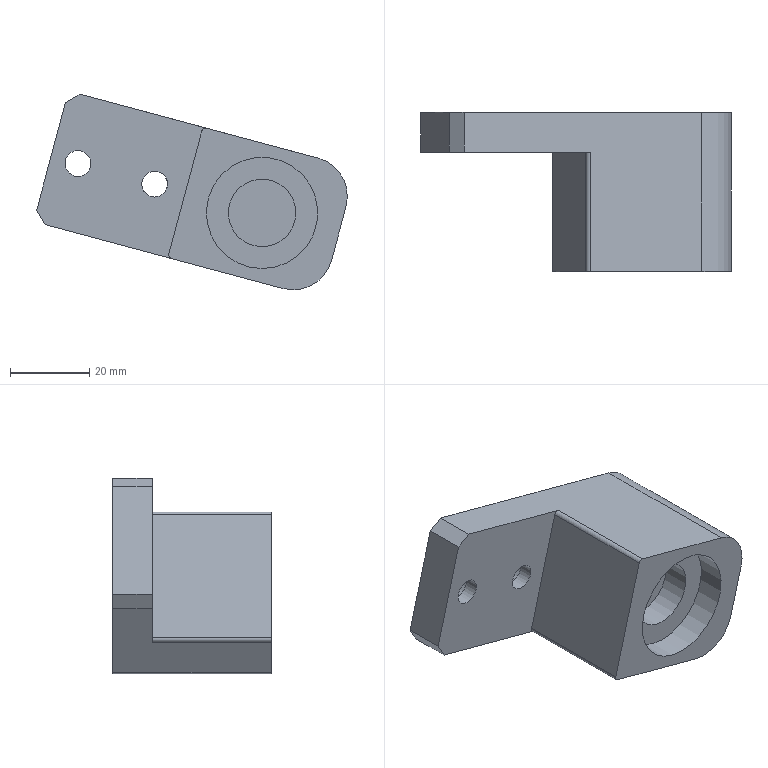CAM job | NX | 3+2 milling, drilling | part box 78.22 x 40 x 49.229 mm | stock box 86.333 x 45 x 54.513 mm
Tools:
number,name,description,diameter,corner_radius,flute_length,length,flutes
6,D6,平底铣刀-粗,6.0,0.0,25.0,75.0,2
9,D10,平底铣刀-粗,10.0,0.0,35.0,75.0,2
7,D6-J,平底铣刀-精,6.0,0.0,25.0,75.0,2
10,D10-J,平底铣刀-精,10.0,0.0,35.0,75.0,2
1,D80R0.8飞刀,圆鼻刀-粗,80.0,0.8,50.0,75.0,2
1,D80R0.8飞刀-J,圆鼻刀-精,80.0,0.8,50.0,75.0,2
2,D6倒角刀,倒角刀,6.0,0.0,3.0,25.0,2
17,ZT6.5,钻头,6.5,0.0,35.0,50.0,2
Operations:
program,operation,operation_type,tool,method,geometry_group,spindle_rpm,surface_speed,feed_per_tooth,feed_cut,feed_plunge,cut_length_mm,path_length_mm,cut_time_min,machine_time_min
B,底壁铣飞面一刀开粗_COPY,VolumeBased25DMillingOperation,D80R0.8飞刀,分层开粗-切深K-步距G,W-B,2800.0,703.696,0.5357,3000.0,100.0,1649.091,3281.618,0.5497,0.7129
B,底壁铣飞面一刀精光_COPY,VolumeBased25DMillingOperation,D80R0.8飞刀-J,侧刃精光-切深K-步距G,W-B,4000.0,1005.28,0.125,1000.0,100.0,183.036,219.036,0.183,0.1866
B,孔粗_3,CylinderMilling,D10,METHOD,W-B,6000.0,157.0,0.25,3000.0,90.0,1411.128,1457.548,0.4706,0.4753
B,底壁铣螺旋开粗-中_COPY,VolumeBased25DMillingOperation,D10,分层开粗-切深K-步距G,W-B,8000.0,251.327,0.125,2000.0,100.0,640.069,698.969,0.32,0.3259
B,底壁铣分层开粗-中_COPY,VolumeBased25DMillingOperation,D10,分层开粗-切深K-步距G,W-B,8000.0,251.32,0.25,4000.0,100.0,13485.815,19348.551,3.372,3.958
B,底壁铣精光底面-中_COPY,VolumeBased25DMillingOperation,D10-J,精光步距切深关,W-B,7000.0,175.0,0.0536,1500.0,100.0,291.651,377.651,0.1944,0.203
B,平面去毛刺6X45L_COPY,SurfaceContour,D6倒角刀,爬面_倒角-切深0-步距G,W-B,6500.0,122.519,0.1154,1500.0,100.0,485.225,889.334,0.3235,0.3639
B,底壁铣精光侧面-中_COPY,VolumeBased25DMillingOperation,D10-J,侧刃精光-切深K-步距G,W-B,8000.0,251.327,0.0375,600.0,100.0,31.858,85.858,0.0531,0.0585
B,底壁铣精光侧面-中_COPY_1,VolumeBased25DMillingOperation,D10-J,侧刃精光-切深K-步距G,W-B,8000.0,251.32,0.0625,1000.0,100.0,65.489,105.489,0.0655,0.0695
B,底壁铣精光侧面-中-选底面_COPY,VolumeBased25DMillingOperation,D10-J,侧刃精光-切深K-步距G,W-B,8000.0,251.32,0.0625,1000.0,100.0,118.07,310.469,0.1181,0.1373
A,顶面,FaceMilling,D80R0.8飞刀,侧刃精光-切深K-步距G,W-A,4000.0,1005.31,0.125,1000.0,100.0,169.0,205.0,0.169,0.1726
A,外形粗_2,VolumeBased25DMillingOperation,D10,METHOD,W-A,8000.0,251.327,0.3125,5000.0,80.0,12612.676,12691.476,2.522,2.53
A,沉头孔打点-深0.8,Operation,D6倒角刀,NONE,W-A,8000.0,150.796,0.0312,500.0,90.0,3.6,68.225,0.0072,0.0137
A,沉头孔-钻孔0段,Operation,ZT6.5,NONE,W-A,1200.0,24.504,0.0625,150.0,90.0,29.906,120.836,0.1994,0.2085
A,铣孔开粗D6_1,CylinderMilling,D6,NONE,W-A,8000.0,150.796,0.075,1200.0,100.0,467.701,579.701,0.3898,0.401
A,铣孔精光D6_1,CylinderMilling,D6-J,精光步距切深关,W-A,8000.0,150.796,0.0312,500.0,100.0,89.89,202.89,0.1798,0.1911
A,仅选体,SurfaceContour,D6倒角刀,METHOD,W-A,8000.0,150.796,0.1875,3000.0,100.0,221.923,257.124,0.074,0.0775
A,铣倒角_1,PlanarMilling,D6倒角刀,NONE,W-A,8000.0,150.796,0.05,800.0,100.0,89.299,179.754,0.1116,0.1207
A,外形半精_2,VolumeBased25DMillingOperation,D10-J,METHOD,W-A,8000.0,251.327,0.0625,1000.0,100.0,726.982,1010.194,0.727,0.7553